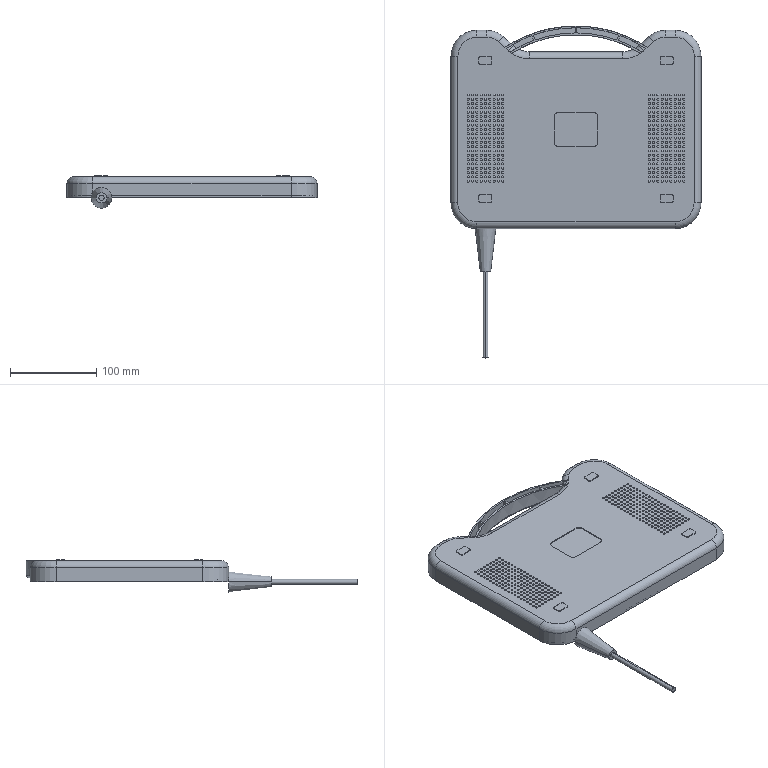Part | STEP file | 11B | 1 solid | 571 faces | box 290 x 385 x 37.5 mm | volume 218260 mm3 | sphere 378 | cylinder 93 | plane 78 | torus 20 | cone 2 | commonest cylinder face diameters 10 x20 4 x16 16 x10 11.6 x8 56 x6 55.6 x4